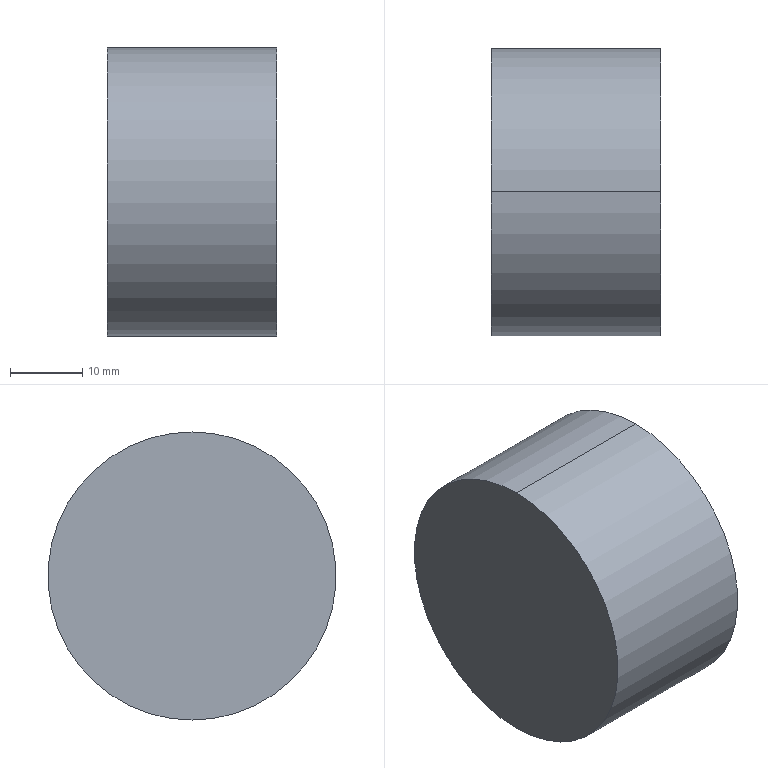Part | SolidWorks | features BaseBody 1 | 1 solid | 4 faces | box 23.5 x 40 x 40 mm | volume 29531 mm3 | cylinder 2 | plane 2 | commonest cylinder face diameters 40 x2
STEP:
#1=CARTESIAN_POINT('',(139.747,459.,-328.));
#2=VERTEX_POINT('',#1);
#3=CARTESIAN_POINT('',(139.747,459.,-368.));
#4=VERTEX_POINT('',#3);
#5=CARTESIAN_POINT('',(139.747,459.,-348.));
#6=DIRECTION('',(-1.,0.,0.));
#7=DIRECTION('',(0.,0.,1.));
#8=AXIS2_PLACEMENT_3D('',#5,#6,#7);
#9=CIRCLE('',#8,20.);
#10=EDGE_CURVE('',#2,#4,#9,.T.);
#11=ORIENTED_EDGE('',*,*,#10,.T.);
#12=CARTESIAN_POINT('',(116.247,459.,-368.));
#13=VERTEX_POINT('',#12);
#14=CARTESIAN_POINT('',(139.747,459.,-368.));
#15=DIRECTION('',(-1.,0.,0.));
#16=VECTOR('',#15,1000.);
#17=LINE('',#14,#16);
#18=EDGE_CURVE('',#4,#13,#17,.T.);
#19=ORIENTED_EDGE('',*,*,#18,.T.);
#20=CARTESIAN_POINT('',(116.247,459.,-328.));
#21=VERTEX_POINT('',#20);
#22=CARTESIAN_POINT('',(116.247,459.,-348.));
#23=DIRECTION('',(1.,0.,0.));
#24=DIRECTION('',(0.,0.,1.));
#25=AXIS2_PLACEMENT_3D('',#22,#23,#24);
#26=CIRCLE('',#25,20.);
#27=EDGE_CURVE('',#13,#21,#26,.T.);
#28=ORIENTED_EDGE('',*,*,#27,.T.);
#29=CARTESIAN_POINT('',(139.747,459.,-328.));
#30=DIRECTION('',(-1.,0.,0.));
#31=VECTOR('',#30,1000.);
#32=LINE('',#29,#31);
#33=EDGE_CURVE('',#2,#21,#32,.T.);
#34=ORIENTED_EDGE('',*,*,#33,.F.);
#35=EDGE_LOOP('',(#11,#19,#28,#34));
#36=FACE_OUTER_BOUND('',#35,.T.);
#37=CARTESIAN_POINT('',(139.747,459.,-348.));
#38=DIRECTION('',(-1.,0.,0.));
#39=DIRECTION('',(0.,0.,1.));
#40=AXIS2_PLACEMENT_3D('',#37,#38,#39);
#41=CYLINDRICAL_SURFACE('',#40,20.);
#42=ADVANCED_FACE('',(#36),#41,.T.);
#43=ORIENTED_EDGE('',*,*,#18,.F.);
#44=CARTESIAN_POINT('',(139.747,459.,-348.));
#45=DIRECTION('',(-1.,0.,0.));
#46=DIRECTION('',(0.,0.,1.));
#47=AXIS2_PLACEMENT_3D('',#44,#45,#46);
#48=CIRCLE('',#47,20.);
#49=EDGE_CURVE('',#4,#2,#48,.T.);
#50=ORIENTED_EDGE('',*,*,#49,.T.);
#51=ORIENTED_EDGE('',*,*,#33,.T.);
#52=CARTESIAN_POINT('',(116.247,459.,-348.));
#53=DIRECTION('',(1.,0.,0.));
#54=DIRECTION('',(0.,0.,1.));
#55=AXIS2_PLACEMENT_3D('',#52,#53,#54);
#56=CIRCLE('',#55,20.);
#57=EDGE_CURVE('',#21,#13,#56,.T.);
#58=ORIENTED_EDGE('',*,*,#57,.T.);
#59=EDGE_LOOP('',(#43,#50,#51,#58));
#60=FACE_OUTER_BOUND('',#59,.T.);
#61=CARTESIAN_POINT('',(139.747,459.,-348.));
#62=DIRECTION('',(-1.,0.,0.));
#63=DIRECTION('',(0.,0.,1.));
#64=AXIS2_PLACEMENT_3D('',#61,#62,#63);
#65=CYLINDRICAL_SURFACE('',#64,20.);
#66=ADVANCED_FACE('',(#60),#65,.T.);
#67=ORIENTED_EDGE('',*,*,#57,.F.);
#68=ORIENTED_EDGE('',*,*,#27,.F.);
#69=EDGE_LOOP('',(#67,#68));
#70=FACE_OUTER_BOUND('',#69,.T.);
#71=CARTESIAN_POINT('',(116.247,419.,-326.));
#72=DIRECTION('',(1.,0.,0.));
#73=DIRECTION('',(0.,0.,-1.));
#74=AXIS2_PLACEMENT_3D('',#71,#72,#73);
#75=PLANE('',#74);
#76=ADVANCED_FACE('',(#70),#75,.F.);
#77=ORIENTED_EDGE('',*,*,#10,.F.);
#78=ORIENTED_EDGE('',*,*,#49,.F.);
#79=EDGE_LOOP('',(#77,#78));
#80=FACE_OUTER_BOUND('',#79,.T.);
#81=CARTESIAN_POINT('',(139.747,459.,-348.));
#82=DIRECTION('',(1.,0.,0.));
#83=DIRECTION('',(0.,0.,-1.));
#84=AXIS2_PLACEMENT_3D('',#81,#82,#83);
#85=PLANE('',#84);
#86=ADVANCED_FACE('',(#80),#85,.T.);
#87=CLOSED_SHELL('',(#42,#66,#76,#86));
#88=MANIFOLD_SOLID_BREP('',#87);
#89=CARTESIAN_POINT('',(0.,0.,0.));
#90=DIRECTION('',(0.,0.,1.));
#91=DIRECTION('',(1.,0.,0.));
#92=AXIS2_PLACEMENT_3D('',#89,#90,#91);
#93=(LENGTH_UNIT()NAMED_UNIT(*)SI_UNIT(.MILLI.,.METRE.));
#94=UNCERTAINTY_MEASURE_WITH_UNIT(LENGTH_MEASURE(0.00001),#93,'','');
#95=(NAMED_UNIT(*)PLANE_ANGLE_UNIT()SI_UNIT($,.RADIAN.));
#96=(NAMED_UNIT(*)SI_UNIT($,.STERADIAN.)SOLID_ANGLE_UNIT());
#97=(GEOMETRIC_REPRESENTATION_CONTEXT(3)GLOBAL_UNCERTAINTY_ASSIGNED_CONTEXT((#94))GLOBAL_UNIT_ASSIGNED_CONTEXT((#93,#95,#96))REPRESENTATION_CONTEXT('',''));
#98=ADVANCED_BREP_SHAPE_REPRESENTATION('',(#88,#92),#97);